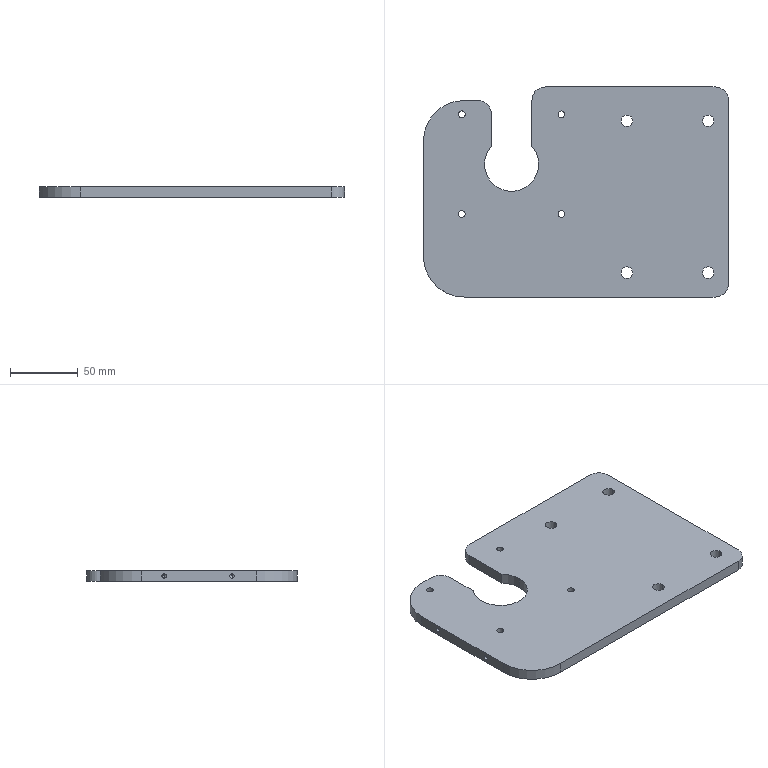Part | SolidWorks | features BaseBody 1 | 1 solid | 42 faces | box 225 x 155 x 8 mm | volume 249145 mm3 | cylinder 29 | plane 9 | cone 4 | commonest cylinder face diameters 5 x8 8.5 x8 3.3 x4 20 x4 40 x3 60 x2
STEP:
#1=CARTESIAN_POINT('',(-67.5,20.5,0.));
#2=VERTEX_POINT('',#1);
#3=CARTESIAN_POINT('',(-27.5,20.5,0.));
#4=VERTEX_POINT('',#3);
#5=CARTESIAN_POINT('',(-47.5,20.5,0.));
#6=DIRECTION('',(0.,0.,1.));
#7=DIRECTION('',(1.,0.,0.));
#8=AXIS2_PLACEMENT_3D('',#5,#6,#7);
#9=CIRCLE('',#8,20.);
#10=EDGE_CURVE('',#2,#4,#9,.T.);
#11=ORIENTED_EDGE('',*,*,#10,.F.);
#12=CARTESIAN_POINT('',(-67.5,20.5,8.));
#13=VERTEX_POINT('',#12);
#14=CARTESIAN_POINT('',(-67.5,20.5,0.));
#15=DIRECTION('',(0.,0.,1.));
#16=VECTOR('',#15,1000.);
#17=LINE('',#14,#16);
#18=EDGE_CURVE('',#2,#13,#17,.T.);
#19=ORIENTED_EDGE('',*,*,#18,.T.);
#20=CARTESIAN_POINT('',(-27.5,20.5,8.));
#21=VERTEX_POINT('',#20);
#22=CARTESIAN_POINT('',(-47.5,20.5,8.));
#23=DIRECTION('',(0.,0.,1.));
#24=DIRECTION('',(1.,0.,0.));
#25=AXIS2_PLACEMENT_3D('',#22,#23,#24);
#26=CIRCLE('',#25,20.);
#27=EDGE_CURVE('',#13,#21,#26,.T.);
#28=ORIENTED_EDGE('',*,*,#27,.T.);
#29=CARTESIAN_POINT('',(-27.5,20.5,0.));
#30=DIRECTION('',(0.,0.,1.));
#31=VECTOR('',#30,1000.);
#32=LINE('',#29,#31);
#33=EDGE_CURVE('',#4,#21,#32,.T.);
#34=ORIENTED_EDGE('',*,*,#33,.F.);
#35=EDGE_LOOP('',(#11,#19,#28,#34));
#36=FACE_OUTER_BOUND('',#35,.T.);
#37=CARTESIAN_POINT('',(-47.5,20.5,0.));
#38=DIRECTION('',(0.,0.,1.));
#39=DIRECTION('',(1.,0.,0.));
#40=AXIS2_PLACEMENT_3D('',#37,#38,#39);
#41=CYLINDRICAL_SURFACE('',#40,20.);
#42=ADVANCED_FACE('',(#36),#41,.F.);
#43=CARTESIAN_POINT('',(-32.5,33.729,0.));
#44=VERTEX_POINT('',#43);
#45=CARTESIAN_POINT('',(-47.5,20.5,0.));
#46=DIRECTION('',(0.,0.,1.));
#47=DIRECTION('',(1.,0.,0.));
#48=AXIS2_PLACEMENT_3D('',#45,#46,#47);
#49=CIRCLE('',#48,20.);
#50=EDGE_CURVE('',#4,#44,#49,.T.);
#51=ORIENTED_EDGE('',*,*,#50,.F.);
#52=ORIENTED_EDGE('',*,*,#33,.T.);
#53=CARTESIAN_POINT('',(-32.5,33.729,8.));
#54=VERTEX_POINT('',#53);
#55=CARTESIAN_POINT('',(-47.5,20.5,8.));
#56=DIRECTION('',(0.,0.,1.));
#57=DIRECTION('',(1.,0.,0.));
#58=AXIS2_PLACEMENT_3D('',#55,#56,#57);
#59=CIRCLE('',#58,20.);
#60=EDGE_CURVE('',#21,#54,#59,.T.);
#61=ORIENTED_EDGE('',*,*,#60,.T.);
#62=CARTESIAN_POINT('',(-32.5,33.729,8.));
#63=DIRECTION('',(0.,0.,-1.));
#64=VECTOR('',#63,1000.);
#65=LINE('',#62,#64);
#66=EDGE_CURVE('',#54,#44,#65,.T.);
#67=ORIENTED_EDGE('',*,*,#66,.T.);
#68=EDGE_LOOP('',(#51,#52,#61,#67));
#69=FACE_OUTER_BOUND('',#68,.T.);
#70=CARTESIAN_POINT('',(-47.5,20.5,0.));
#71=DIRECTION('',(0.,0.,1.));
#72=DIRECTION('',(1.,0.,0.));
#73=AXIS2_PLACEMENT_3D('',#70,#71,#72);
#74=CYLINDRICAL_SURFACE('',#73,20.);
#75=ADVANCED_FACE('',(#69),#74,.F.);
#76=CARTESIAN_POINT('',(33.25,52.5,8.));
#77=VERTEX_POINT('',#76);
#78=CARTESIAN_POINT('',(41.75,52.5,8.));
#79=VERTEX_POINT('',#78);
#80=CARTESIAN_POINT('',(37.5,52.5,8.));
#81=DIRECTION('',(0.,0.,1.));
#82=DIRECTION('',(-1.,0.,0.));
#83=AXIS2_PLACEMENT_3D('',#80,#81,#82);
#84=CIRCLE('',#83,4.25);
#85=EDGE_CURVE('',#77,#79,#84,.T.);
#86=ORIENTED_EDGE('',*,*,#85,.T.);
#87=CARTESIAN_POINT('',(41.75,52.5,0.));
#88=VERTEX_POINT('',#87);
#89=CARTESIAN_POINT('',(41.75,52.5,0.));
#90=DIRECTION('',(0.,0.,-1.));
#91=VECTOR('',#90,1000.);
#92=LINE('',#89,#91);
#93=EDGE_CURVE('',#79,#88,#92,.T.);
#94=ORIENTED_EDGE('',*,*,#93,.T.);
#95=CARTESIAN_POINT('',(33.25,52.5,0.));
#96=VERTEX_POINT('',#95);
#97=CARTESIAN_POINT('',(37.5,52.5,0.));
#98=DIRECTION('',(0.,0.,1.));
#99=DIRECTION('',(-1.,0.,0.));
#100=AXIS2_PLACEMENT_3D('',#97,#98,#99);
#101=CIRCLE('',#100,4.25);
#102=EDGE_CURVE('',#96,#88,#101,.T.);
#103=ORIENTED_EDGE('',*,*,#102,.F.);
#104=CARTESIAN_POINT('',(33.25,52.5,0.));
#105=DIRECTION('',(0.,0.,-1.));
#106=VECTOR('',#105,1000.);
#107=LINE('',#104,#106);
#108=EDGE_CURVE('',#77,#96,#107,.T.);
#109=ORIENTED_EDGE('',*,*,#108,.F.);
#110=EDGE_LOOP('',(#86,#94,#103,#109));
#111=FACE_OUTER_BOUND('',#110,.T.);
#112=CARTESIAN_POINT('',(37.5,52.5,0.));
#113=DIRECTION('',(0.,0.,-1.));
#114=DIRECTION('',(-1.,0.,0.));
#115=AXIS2_PLACEMENT_3D('',#112,#113,#114);
#116=CYLINDRICAL_SURFACE('',#115,4.25);
#117=ADVANCED_FACE('',(#111),#116,.F.);
#118=CARTESIAN_POINT('',(93.25,-59.5,8.));
#119=VERTEX_POINT('',#118);
#120=CARTESIAN_POINT('',(101.75,-59.5,8.));
#121=VERTEX_POINT('',#120);
#122=CARTESIAN_POINT('',(97.5,-59.5,8.));
#123=DIRECTION('',(0.,0.,1.));
#124=DIRECTION('',(-1.,0.,0.));
#125=AXIS2_PLACEMENT_3D('',#122,#123,#124);
#126=CIRCLE('',#125,4.25);
#127=EDGE_CURVE('',#119,#121,#126,.T.);
#128=ORIENTED_EDGE('',*,*,#127,.T.);
#129=CARTESIAN_POINT('',(101.75,-59.5,0.));
#130=VERTEX_POINT('',#129);
#131=CARTESIAN_POINT('',(101.75,-59.5,0.));
#132=DIRECTION('',(0.,0.,-1.));
#133=VECTOR('',#132,1000.);
#134=LINE('',#131,#133);
#135=EDGE_CURVE('',#121,#130,#134,.T.);
#136=ORIENTED_EDGE('',*,*,#135,.T.);
#137=CARTESIAN_POINT('',(93.25,-59.5,0.));
#138=VERTEX_POINT('',#137);
#139=CARTESIAN_POINT('',(97.5,-59.5,0.));
#140=DIRECTION('',(0.,0.,1.));
#141=DIRECTION('',(-1.,0.,0.));
#142=AXIS2_PLACEMENT_3D('',#139,#140,#141);
#143=CIRCLE('',#142,4.25);
#144=EDGE_CURVE('',#138,#130,#143,.T.);
#145=ORIENTED_EDGE('',*,*,#144,.F.);
#146=CARTESIAN_POINT('',(93.25,-59.5,0.));
#147=DIRECTION('',(0.,0.,-1.));
#148=VECTOR('',#147,1000.);
#149=LINE('',#146,#148);
#150=EDGE_CURVE('',#119,#138,#149,.T.);
#151=ORIENTED_EDGE('',*,*,#150,.F.);
#152=EDGE_LOOP('',(#128,#136,#145,#151));
#153=FACE_OUTER_BOUND('',#152,.T.);
#154=CARTESIAN_POINT('',(97.5,-59.5,0.));
#155=DIRECTION('',(0.,0.,-1.));
#156=DIRECTION('',(-1.,0.,0.));
#157=AXIS2_PLACEMENT_3D('',#154,#155,#156);
#158=CYLINDRICAL_SURFACE('',#157,4.25);
#159=ADVANCED_FACE('',(#153),#158,.F.);
#160=CARTESIAN_POINT('',(33.25,-59.5,8.));
#161=VERTEX_POINT('',#160);
#162=CARTESIAN_POINT('',(41.75,-59.5,8.));
#163=VERTEX_POINT('',#162);
#164=CARTESIAN_POINT('',(37.5,-59.5,8.));
#165=DIRECTION('',(0.,0.,1.));
#166=DIRECTION('',(-1.,0.,0.));
#167=AXIS2_PLACEMENT_3D('',#164,#165,#166);
#168=CIRCLE('',#167,4.25);
#169=EDGE_CURVE('',#161,#163,#168,.T.);
#170=ORIENTED_EDGE('',*,*,#169,.T.);
#171=CARTESIAN_POINT('',(41.75,-59.5,0.));
#172=VERTEX_POINT('',#171);
#173=CARTESIAN_POINT('',(41.75,-59.5,0.));
#174=DIRECTION('',(0.,0.,-1.));
#175=VECTOR('',#174,1000.);
#176=LINE('',#173,#175);
#177=EDGE_CURVE('',#163,#172,#176,.T.);
#178=ORIENTED_EDGE('',*,*,#177,.T.);
#179=CARTESIAN_POINT('',(33.25,-59.5,0.));
#180=VERTEX_POINT('',#179);
#181=CARTESIAN_POINT('',(37.5,-59.5,0.));
#182=DIRECTION('',(0.,0.,1.));
#183=DIRECTION('',(-1.,0.,0.));
#184=AXIS2_PLACEMENT_3D('',#181,#182,#183);
#185=CIRCLE('',#184,4.25);
#186=EDGE_CURVE('',#180,#172,#185,.T.);
#187=ORIENTED_EDGE('',*,*,#186,.F.);
#188=CARTESIAN_POINT('',(33.25,-59.5,0.));
#189=DIRECTION('',(0.,0.,-1.));
#190=VECTOR('',#189,1000.);
#191=LINE('',#188,#190);
#192=EDGE_CURVE('',#161,#180,#191,.T.);
#193=ORIENTED_EDGE('',*,*,#192,.F.);
#194=EDGE_LOOP('',(#170,#178,#187,#193));
#195=FACE_OUTER_BOUND('',#194,.T.);
#196=CARTESIAN_POINT('',(37.5,-59.5,0.));
#197=DIRECTION('',(0.,0.,-1.));
#198=DIRECTION('',(-1.,0.,0.));
#199=AXIS2_PLACEMENT_3D('',#196,#197,#198);
#200=CYLINDRICAL_SURFACE('',#199,4.25);
#201=ADVANCED_FACE('',(#195),#200,.F.);
#202=CARTESIAN_POINT('',(93.25,52.5,8.));
#203=VERTEX_POINT('',#202);
#204=CARTESIAN_POINT('',(101.75,52.5,8.));
#205=VERTEX_POINT('',#204);
#206=CARTESIAN_POINT('',(97.5,52.5,8.));
#207=DIRECTION('',(0.,0.,1.));
#208=DIRECTION('',(-1.,0.,0.));
#209=AXIS2_PLACEMENT_3D('',#206,#207,#208);
#210=CIRCLE('',#209,4.25);
#211=EDGE_CURVE('',#203,#205,#210,.T.);
#212=ORIENTED_EDGE('',*,*,#211,.T.);
#213=CARTESIAN_POINT('',(101.75,52.5,0.));
#214=VERTEX_POINT('',#213);
#215=CARTESIAN_POINT('',(101.75,52.5,0.));
#216=DIRECTION('',(0.,0.,-1.));
#217=VECTOR('',#216,1000.);
#218=LINE('',#215,#217);
#219=EDGE_CURVE('',#205,#214,#218,.T.);
#220=ORIENTED_EDGE('',*,*,#219,.T.);
#221=CARTESIAN_POINT('',(93.25,52.5,0.));
#222=VERTEX_POINT('',#221);
#223=CARTESIAN_POINT('',(97.5,52.5,0.));
#224=DIRECTION('',(0.,0.,1.));
#225=DIRECTION('',(-1.,0.,0.));
#226=AXIS2_PLACEMENT_3D('',#223,#224,#225);
#227=CIRCLE('',#226,4.25);
#228=EDGE_CURVE('',#222,#214,#227,.T.);
#229=ORIENTED_EDGE('',*,*,#228,.F.);
#230=CARTESIAN_POINT('',(93.25,52.5,0.));
#231=DIRECTION('',(0.,0.,-1.));
#232=VECTOR('',#231,1000.);
#233=LINE('',#230,#232);
#234=EDGE_CURVE('',#203,#222,#233,.T.);
#235=ORIENTED_EDGE('',*,*,#234,.F.);
#236=EDGE_LOOP('',(#212,#220,#229,#235));
#237=FACE_OUTER_BOUND('',#236,.T.);
#238=CARTESIAN_POINT('',(97.5,52.5,0.));
#239=DIRECTION('',(0.,0.,-1.));
#240=DIRECTION('',(-1.,0.,0.));
#241=AXIS2_PLACEMENT_3D('',#238,#239,#240);
#242=CYLINDRICAL_SURFACE('',#241,4.25);
#243=ADVANCED_FACE('',(#237),#242,.F.);
#244=CARTESIAN_POINT('',(-86.77,57.27,8.));
#245=VERTEX_POINT('',#244);
#246=CARTESIAN_POINT('',(-81.77,57.27,8.));
#247=VERTEX_POINT('',#246);
#248=CARTESIAN_POINT('',(-84.27,57.27,8.));
#249=DIRECTION('',(0.,0.,1.));
#250=DIRECTION('',(-1.,0.,0.));
#251=AXIS2_PLACEMENT_3D('',#248,#249,#250);
#252=CIRCLE('',#251,2.5);
#253=EDGE_CURVE('',#245,#247,#252,.T.);
#254=ORIENTED_EDGE('',*,*,#253,.T.);
#255=CARTESIAN_POINT('',(-81.77,57.27,0.));
#256=VERTEX_POINT('',#255);
#257=CARTESIAN_POINT('',(-81.77,57.27,0.));
#258=DIRECTION('',(0.,0.,-1.));
#259=VECTOR('',#258,1000.);
#260=LINE('',#257,#259);
#261=EDGE_CURVE('',#247,#256,#260,.T.);
#262=ORIENTED_EDGE('',*,*,#261,.T.);
#263=CARTESIAN_POINT('',(-86.77,57.27,0.));
#264=VERTEX_POINT('',#263);
#265=CARTESIAN_POINT('',(-84.27,57.27,0.));
#266=DIRECTION('',(0.,0.,1.));
#267=DIRECTION('',(-1.,0.,0.));
#268=AXIS2_PLACEMENT_3D('',#265,#266,#267);
#269=CIRCLE('',#268,2.5);
#270=EDGE_CURVE('',#264,#256,#269,.T.);
#271=ORIENTED_EDGE('',*,*,#270,.F.);
#272=CARTESIAN_POINT('',(-86.77,57.27,0.));
#273=DIRECTION('',(0.,0.,-1.));
#274=VECTOR('',#273,1000.);
#275=LINE('',#272,#274);
#276=EDGE_CURVE('',#245,#264,#275,.T.);
#277=ORIENTED_EDGE('',*,*,#276,.F.);
#278=EDGE_LOOP('',(#254,#262,#271,#277));
#279=FACE_OUTER_BOUND('',#278,.T.);
#280=CARTESIAN_POINT('',(-84.27,57.27,0.));
#281=DIRECTION('',(0.,0.,-1.));
#282=DIRECTION('',(-1.,0.,0.));
#283=AXIS2_PLACEMENT_3D('',#280,#281,#282);
#284=CYLINDRICAL_SURFACE('',#283,2.5);
#285=ADVANCED_FACE('',(#279),#284,.F.);
#286=CARTESIAN_POINT('',(-13.23,-16.27,8.));
#287=VERTEX_POINT('',#286);
#288=CARTESIAN_POINT('',(-8.23,-16.27,8.));
#289=VERTEX_POINT('',#288);
#290=CARTESIAN_POINT('',(-10.73,-16.27,8.));
#291=DIRECTION('',(0.,0.,1.));
#292=DIRECTION('',(-1.,0.,0.));
#293=AXIS2_PLACEMENT_3D('',#290,#291,#292);
#294=CIRCLE('',#293,2.5);
#295=EDGE_CURVE('',#287,#289,#294,.T.);
#296=ORIENTED_EDGE('',*,*,#295,.T.);
#297=CARTESIAN_POINT('',(-8.23,-16.27,0.));
#298=VERTEX_POINT('',#297);
#299=CARTESIAN_POINT('',(-8.23,-16.27,0.));
#300=DIRECTION('',(0.,0.,-1.));
#301=VECTOR('',#300,1000.);
#302=LINE('',#299,#301);
#303=EDGE_CURVE('',#289,#298,#302,.T.);
#304=ORIENTED_EDGE('',*,*,#303,.T.);
#305=CARTESIAN_POINT('',(-13.23,-16.27,0.));
#306=VERTEX_POINT('',#305);
#307=CARTESIAN_POINT('',(-10.73,-16.27,0.));
#308=DIRECTION('',(0.,0.,1.));
#309=DIRECTION('',(-1.,0.,0.));
#310=AXIS2_PLACEMENT_3D('',#307,#308,#309);
#311=CIRCLE('',#310,2.5);
#312=EDGE_CURVE('',#306,#298,#311,.T.);
#313=ORIENTED_EDGE('',*,*,#312,.F.);
#314=CARTESIAN_POINT('',(-13.23,-16.27,0.));
#315=DIRECTION('',(0.,0.,-1.));
#316=VECTOR('',#315,1000.);
#317=LINE('',#314,#316);
#318=EDGE_CURVE('',#287,#306,#317,.T.);
#319=ORIENTED_EDGE('',*,*,#318,.F.);
#320=EDGE_LOOP('',(#296,#304,#313,#319));
#321=FACE_OUTER_BOUND('',#320,.T.);
#322=CARTESIAN_POINT('',(-10.73,-16.27,0.));
#323=DIRECTION('',(0.,0.,-1.));
#324=DIRECTION('',(-1.,0.,0.));
#325=AXIS2_PLACEMENT_3D('',#322,#323,#324);
#326=CYLINDRICAL_SURFACE('',#325,2.5);
#327=ADVANCED_FACE('',(#321),#326,.F.);
#328=CARTESIAN_POINT('',(-13.23,57.27,8.));
#329=VERTEX_POINT('',#328);
#330=CARTESIAN_POINT('',(-8.23,57.27,8.));
#331=VERTEX_POINT('',#330);
#332=CARTESIAN_POINT('',(-10.73,57.27,8.));
#333=DIRECTION('',(0.,0.,1.));
#334=DIRECTION('',(-1.,0.,0.));
#335=AXIS2_PLACEMENT_3D('',#332,#333,#334);
#336=CIRCLE('',#335,2.5);
#337=EDGE_CURVE('',#329,#331,#336,.T.);
#338=ORIENTED_EDGE('',*,*,#337,.T.);
#339=CARTESIAN_POINT('',(-8.23,57.27,0.));
#340=VERTEX_POINT('',#339);
#341=CARTESIAN_POINT('',(-8.23,57.27,0.));
#342=DIRECTION('',(0.,0.,-1.));
#343=VECTOR('',#342,1000.);
#344=LINE('',#341,#343);
#345=EDGE_CURVE('',#331,#340,#344,.T.);
#346=ORIENTED_EDGE('',*,*,#345,.T.);
#347=CARTESIAN_POINT('',(-13.23,57.27,0.));
#348=VERTEX_POINT('',#347);
#349=CARTESIAN_POINT('',(-10.73,57.27,0.));
#350=DIRECTION('',(0.,0.,1.));
#351=DIRECTION('',(-1.,0.,0.));
#352=AXIS2_PLACEMENT_3D('',#349,#350,#351);
#353=CIRCLE('',#352,2.5);
#354=EDGE_CURVE('',#348,#340,#353,.T.);
#355=ORIENTED_EDGE('',*,*,#354,.F.);
#356=CARTESIAN_POINT('',(-13.23,57.27,0.));
#357=DIRECTION('',(0.,0.,-1.));
#358=VECTOR('',#357,1000.);
#359=LINE('',#356,#358);
#360=EDGE_CURVE('',#329,#348,#359,.T.);
#361=ORIENTED_EDGE('',*,*,#360,.F.);
#362=EDGE_LOOP('',(#338,#346,#355,#361));
#363=FACE_OUTER_BOUND('',#362,.T.);
#364=CARTESIAN_POINT('',(-10.73,57.27,0.));
#365=DIRECTION('',(0.,0.,-1.));
#366=DIRECTION('',(-1.,0.,0.));
#367=AXIS2_PLACEMENT_3D('',#364,#365,#366);
#368=CYLINDRICAL_SURFACE('',#367,2.5);
#369=ADVANCED_FACE('',(#363),#368,.F.);
#370=CARTESIAN_POINT('',(-86.77,-16.27,8.));
#371=VERTEX_POINT('',#370);
#372=CARTESIAN_POINT('',(-81.77,-16.27,8.));
#373=VERTEX_POINT('',#372);
#374=CARTESIAN_POINT('',(-84.27,-16.27,8.));
#375=DIRECTION('',(0.,0.,1.));
#376=DIRECTION('',(-1.,0.,0.));
#377=AXIS2_PLACEMENT_3D('',#374,#375,#376);
#378=CIRCLE('',#377,2.5);
#379=EDGE_CURVE('',#371,#373,#378,.T.);
#380=ORIENTED_EDGE('',*,*,#379,.T.);
#381=CARTESIAN_POINT('',(-81.77,-16.27,0.));
#382=VERTEX_POINT('',#381);
#383=CARTESIAN_POINT('',(-81.77,-16.27,0.));
#384=DIRECTION('',(0.,0.,-1.));
#385=VECTOR('',#384,1000.);
#386=LINE('',#383,#385);
#387=EDGE_CURVE('',#373,#382,#386,.T.);
#388=ORIENTED_EDGE('',*,*,#387,.T.);
#389=CARTESIAN_POINT('',(-86.77,-16.27,0.));
#390=VERTEX_POINT('',#389);
#391=CARTESIAN_POINT('',(-84.27,-16.27,0.));
#392=DIRECTION('',(0.,0.,1.));
#393=DIRECTION('',(-1.,0.,0.));
#394=AXIS2_PLACEMENT_3D('',#391,#392,#393);
#395=CIRCLE('',#394,2.5);
#396=EDGE_CURVE('',#390,#382,#395,.T.);
#397=ORIENTED_EDGE('',*,*,#396,.F.);
#398=CARTESIAN_POINT('',(-86.77,-16.27,0.));
#399=DIRECTION('',(0.,0.,-1.));
#400=VECTOR('',#399,1000.);
#401=LINE('',#398,#400);
#402=EDGE_CURVE('',#371,#390,#401,.T.);
#403=ORIENTED_EDGE('',*,*,#402,.F.);
#404=EDGE_LOOP('',(#380,#388,#397,#403));
#405=FACE_OUTER_BOUND('',#404,.T.);
#406=CARTESIAN_POINT('',(-84.27,-16.27,0.));
#407=DIRECTION('',(0.,0.,-1.));
#408=DIRECTION('',(-1.,0.,0.));
#409=AXIS2_PLACEMENT_3D('',#406,#407,#408);
#410=CYLINDRICAL_SURFACE('',#409,2.5);
#411=ADVANCED_FACE('',(#405),#410,.F.);
#412=CARTESIAN_POINT('',(-101.,20.5,2.35));
#413=VERTEX_POINT('',#412);
#414=CARTESIAN_POINT('',(-101.,20.5,5.65));
#415=VERTEX_POINT('',#414);
#416=CARTESIAN_POINT('',(-101.,20.5,4.));
#417=DIRECTION('',(-1.,0.,0.));
#418=DIRECTION('',(0.,0.,1.));
#419=AXIS2_PLACEMENT_3D('',#416,#417,#418);
#420=CIRCLE('',#419,1.65);
#421=EDGE_CURVE('',#413,#415,#420,.T.);
#422=ORIENTED_EDGE('',*,*,#421,.F.);
#423=CARTESIAN_POINT('',(-112.5,20.5,2.35));
#424=VERTEX_POINT('',#423);
#425=CARTESIAN_POINT('',(-112.5,20.5,2.35));
#426=DIRECTION('',(-1.,0.,0.));
#427=VECTOR('',#426,1000.);
#428=LINE('',#425,#427);
#429=EDGE_CURVE('',#413,#424,#428,.T.);
#430=ORIENTED_EDGE('',*,*,#429,.T.);
#431=CARTESIAN_POINT('',(-112.5,20.5,5.65));
#432=VERTEX_POINT('',#431);
#433=CARTESIAN_POINT('',(-112.5,20.5,4.));
#434=DIRECTION('',(-1.,0.,0.));
#435=DIRECTION('',(0.,0.,1.));
#436=AXIS2_PLACEMENT_3D('',#433,#434,#435);
#437=CIRCLE('',#436,1.65);
#438=EDGE_CURVE('',#424,#432,#437,.T.);
#439=ORIENTED_EDGE('',*,*,#438,.T.);
#440=CARTESIAN_POINT('',(-112.5,20.5,5.65));
#441=DIRECTION('',(-1.,0.,0.));
#442=VECTOR('',#441,1000.);
#443=LINE('',#440,#442);
#444=EDGE_CURVE('',#415,#432,#443,.T.);
#445=ORIENTED_EDGE('',*,*,#444,.F.);
#446=EDGE_LOOP('',(#422,#430,#439,#445));
#447=FACE_OUTER_BOUND('',#446,.T.);
#448=CARTESIAN_POINT('',(-112.5,20.5,4.));
#449=DIRECTION('',(-1.,0.,0.));
#450=DIRECTION('',(0.,0.,1.));
#451=AXIS2_PLACEMENT_3D('',#448,#449,#450);
#452=CYLINDRICAL_SURFACE('',#451,1.65);
#453=ADVANCED_FACE('',(#447),#452,.F.);
#454=CARTESIAN_POINT('',(-101.,-29.5,2.35));
#455=VERTEX_POINT('',#454);
#456=CARTESIAN_POINT('',(-101.,-29.5,5.65));
#457=VERTEX_POINT('',#456);
#458=CARTESIAN_POINT('',(-101.,-29.5,4.));
#459=DIRECTION('',(-1.,0.,0.));
#460=DIRECTION('',(0.,0.,1.));
#461=AXIS2_PLACEMENT_3D('',#458,#459,#460);
#462=CIRCLE('',#461,1.65);
#463=EDGE_CURVE('',#455,#457,#462,.T.);
#464=ORIENTED_EDGE('',*,*,#463,.F.);
#465=CARTESIAN_POINT('',(-112.5,-29.5,2.35));
#466=VERTEX_POINT('',#465);
#467=CARTESIAN_POINT('',(-112.5,-29.5,2.35));
#468=DIRECTION('',(-1.,0.,0.));
#469=VECTOR('',#468,1000.);
#470=LINE('',#467,#469);
#471=EDGE_CURVE('',#455,#466,#470,.T.);
#472=ORIENTED_EDGE('',*,*,#471,.T.);
#473=CARTESIAN_POINT('',(-112.5,-29.5,5.65));
#474=VERTEX_POINT('',#473);
#475=CARTESIAN_POINT('',(-112.5,-29.5,4.));
#476=DIRECTION('',(-1.,0.,0.));
#477=DIRECTION('',(0.,0.,1.));
#478=AXIS2_PLACEMENT_3D('',#475,#476,#477);
#479=CIRCLE('',#478,1.65);
#480=EDGE_CURVE('',#466,#474,#479,.T.);
#481=ORIENTED_EDGE('',*,*,#480,.T.);
#482=CARTESIAN_POINT('',(-112.5,-29.5,5.65));
#483=DIRECTION('',(-1.,0.,0.));
#484=VECTOR('',#483,1000.);
#485=LINE('',#482,#484);
#486=EDGE_CURVE('',#457,#474,#485,.T.);
#487=ORIENTED_EDGE('',*,*,#486,.F.);
#488=EDGE_LOOP('',(#464,#472,#481,#487));
#489=FACE_OUTER_BOUND('',#488,.T.);
#490=CARTESIAN_POINT('',(-112.5,-29.5,4.));
#491=DIRECTION('',(-1.,0.,0.));
#492=DIRECTION('',(0.,0.,1.));
#493=AXIS2_PLACEMENT_3D('',#490,#491,#492);
#494=CYLINDRICAL_SURFACE('',#493,1.65);
#495=ADVANCED_FACE('',(#489),#494,.F.);
#496=CARTESIAN_POINT('',(-100.009,20.5,4.));
#497=VERTEX_POINT('',#496);
#498=CARTESIAN_POINT('',(-101.,20.5,5.65));
#499=DIRECTION('',(-0.515,0.,0.8572));
#500=VECTOR('',#499,1000.);
#501=LINE('',#498,#500);
#502=EDGE_CURVE('',#497,#415,#501,.T.);
#503=ORIENTED_EDGE('',*,*,#502,.F.);
#504=CARTESIAN_POINT('',(-101.,20.5,2.35));
#505=DIRECTION('',(-0.515,0.,-0.8572));
#506=VECTOR('',#505,1000.);
#507=LINE('',#504,#506);
#508=EDGE_CURVE('',#497,#413,#507,.T.);
#509=ORIENTED_EDGE('',*,*,#508,.T.);
#510=ORIENTED_EDGE('',*,*,#421,.T.);
#511=EDGE_LOOP('',(#503,#509,#510));
#512=FACE_OUTER_BOUND('',#511,.T.);
#513=CARTESIAN_POINT('',(-101.,20.5,4.));
#514=DIRECTION('',(-1.,0.,0.));
#515=DIRECTION('',(0.,0.,1.));
#516=AXIS2_PLACEMENT_3D('',#513,#514,#515);
#517=CONICAL_SURFACE('',#516,1.65,1.03);
#518=ADVANCED_FACE('',(#512),#517,.F.);
#519=CARTESIAN_POINT('',(-100.009,-29.5,4.));
#520=VERTEX_POINT('',#519);
#521=CARTESIAN_POINT('',(-101.,-29.5,5.65));
#522=DIRECTION('',(-0.515,0.,0.8572));
#523=VECTOR('',#522,1000.);
#524=LINE('',#521,#523);
#525=EDGE_CURVE('',#520,#457,#524,.T.);
#526=ORIENTED_EDGE('',*,*,#525,.F.);
#527=CARTESIAN_POINT('',(-101.,-29.5,2.35));
#528=DIRECTION('',(-0.515,0.,-0.8572));
#529=VECTOR('',#528,1000.);
#530=LINE('',#527,#529);
#531=EDGE_CURVE('',#520,#455,#530,.T.);
#532=ORIENTED_EDGE('',*,*,#531,.T.);
#533=ORIENTED_EDGE('',*,*,#463,.T.);
#534=EDGE_LOOP('',(#526,#532,#533));
#535=FACE_OUTER_BOUND('',#534,.T.);
#536=CARTESIAN_POINT('',(-101.,-29.5,4.));
#537=DIRECTION('',(-1.,0.,0.));
#538=DIRECTION('',(0.,0.,1.));
#539=AXIS2_PLACEMENT_3D('',#536,#537,#538);
#540=CONICAL_SURFACE('',#539,1.65,1.03);
#541=ADVANCED_FACE('',(#535),#540,.F.);
#542=CARTESIAN_POINT('',(102.5,77.5,8.));
#543=VERTEX_POINT('',#542);
#544=CARTESIAN_POINT('',(112.5,67.5,8.));
#545=VERTEX_POINT('',#544);
#546=CARTESIAN_POINT('',(102.5,67.5,8.));
#547=DIRECTION('',(0.,0.,-1.));
#548=DIRECTION('',(-1.,0.,0.));
#549=AXIS2_PLACEMENT_3D('',#546,#547,#548);
#550=CIRCLE('',#549,10.);
#551=EDGE_CURVE('',#543,#545,#550,.T.);
#552=ORIENTED_EDGE('',*,*,#551,.F.);
#553=CARTESIAN_POINT('',(-22.5,77.5,8.));
#554=VERTEX_POINT('',#553);
#555=CARTESIAN_POINT('',(0.,77.5,8.));
#556=DIRECTION('',(1.,0.,0.));
#557=VECTOR('',#556,1000.);
#558=LINE('',#555,#557);
#559=EDGE_CURVE('',#554,#543,#558,.T.);
#560=ORIENTED_EDGE('',*,*,#559,.F.);
#561=CARTESIAN_POINT('',(-32.5,67.5,8.));
#562=VERTEX_POINT('',#561);
#563=CARTESIAN_POINT('',(-22.5,67.5,8.));
#564=DIRECTION('',(0.,0.,-1.));
#565=DIRECTION('',(1.,0.,0.));
#566=AXIS2_PLACEMENT_3D('',#563,#564,#565);
#567=CIRCLE('',#566,10.);
#568=EDGE_CURVE('',#562,#554,#567,.T.);
#569=ORIENTED_EDGE('',*,*,#568,.F.);
#570=CARTESIAN_POINT('',(-32.5,0.,8.));
#571=DIRECTION('',(0.,1.,0.));
#572=VECTOR('',#571,1000.);
#573=LINE('',#570,#572);
#574=EDGE_CURVE('',#54,#562,#573,.T.);
#575=ORIENTED_EDGE('',*,*,#574,.F.);
#576=ORIENTED_EDGE('',*,*,#60,.F.);
#577=ORIENTED_EDGE('',*,*,#27,.F.);
#578=CARTESIAN_POINT('',(-62.5,33.729,8.));
#579=VERTEX_POINT('',#578);
#580=CARTESIAN_POINT('',(-47.5,20.5,8.));
#581=DIRECTION('',(0.,0.,1.));
#582=DIRECTION('',(1.,0.,0.));
#583=AXIS2_PLACEMENT_3D('',#580,#581,#582);
#584=CIRCLE('',#583,20.);
#585=EDGE_CURVE('',#579,#13,#584,.T.);
#586=ORIENTED_EDGE('',*,*,#585,.F.);
#587=CARTESIAN_POINT('',(-62.5,57.5,8.));
#588=VERTEX_POINT('',#587);
#589=CARTESIAN_POINT('',(-62.5,0.,8.));
#590=DIRECTION('',(0.,-1.,0.));
#591=VECTOR('',#590,1000.);
#592=LINE('',#589,#591);
#593=EDGE_CURVE('',#588,#579,#592,.T.);
#594=ORIENTED_EDGE('',*,*,#593,.F.);
#595=CARTESIAN_POINT('',(-72.5,67.5,8.));
#596=VERTEX_POINT('',#595);
#597=CARTESIAN_POINT('',(-72.5,57.5,8.));
#598=DIRECTION('',(0.,0.,-1.));
#599=DIRECTION('',(1.,0.,0.));
#600=AXIS2_PLACEMENT_3D('',#597,#598,#599);
#601=CIRCLE('',#600,10.);
#602=EDGE_CURVE('',#596,#588,#601,.T.);
#603=ORIENTED_EDGE('',*,*,#602,.F.);
#604=CARTESIAN_POINT('',(-82.5,67.5,8.));
#605=VERTEX_POINT('',#604);
#606=CARTESIAN_POINT('',(0.,67.5,8.));
#607=DIRECTION('',(1.,0.,0.));
#608=VECTOR('',#607,1000.);
#609=LINE('',#606,#608);
#610=EDGE_CURVE('',#605,#596,#609,.T.);
#611=ORIENTED_EDGE('',*,*,#610,.F.);
#612=CARTESIAN_POINT('',(-112.5,37.5,8.));
#613=VERTEX_POINT('',#612);
#614=CARTESIAN_POINT('',(-82.5,37.5,8.));
#615=DIRECTION('',(0.,0.,-1.));
#616=DIRECTION('',(1.,0.,0.));
#617=AXIS2_PLACEMENT_3D('',#614,#615,#616);
#618=CIRCLE('',#617,30.);
#619=EDGE_CURVE('',#613,#605,#618,.T.);
#620=ORIENTED_EDGE('',*,*,#619,.F.);
#621=CARTESIAN_POINT('',(-112.5,-47.5,8.));
#622=VERTEX_POINT('',#621);
#623=CARTESIAN_POINT('',(-112.5,0.,8.));
#624=DIRECTION('',(0.,1.,0.));
#625=VECTOR('',#624,1000.);
#626=LINE('',#623,#625);
#627=EDGE_CURVE('',#622,#613,#626,.T.);
#628=ORIENTED_EDGE('',*,*,#627,.F.);
#629=CARTESIAN_POINT('',(-82.5,-77.5,8.));
#630=VERTEX_POINT('',#629);
#631=CARTESIAN_POINT('',(-82.5,-47.5,8.));
#632=DIRECTION('',(0.,0.,-1.));
#633=DIRECTION('',(-1.,0.,0.));
#634=AXIS2_PLACEMENT_3D('',#631,#632,#633);
#635=CIRCLE('',#634,30.);
#636=EDGE_CURVE('',#630,#622,#635,.T.);
#637=ORIENTED_EDGE('',*,*,#636,.F.);
#638=CARTESIAN_POINT('',(102.5,-77.5,8.));
#639=VERTEX_POINT('',#638);
#640=CARTESIAN_POINT('',(0.,-77.5,8.));
#641=DIRECTION('',(-1.,0.,0.));
#642=VECTOR('',#641,1000.);
#643=LINE('',#640,#642);
#644=EDGE_CURVE('',#639,#630,#643,.T.);
#645=ORIENTED_EDGE('',*,*,#644,.F.);
#646=CARTESIAN_POINT('',(112.5,-67.5,8.));
#647=VERTEX_POINT('',#646);
#648=CARTESIAN_POINT('',(102.5,-67.5,8.));
#649=DIRECTION('',(0.,0.,-1.));
#650=DIRECTION('',(-1.,0.,0.));
#651=AXIS2_PLACEMENT_3D('',#648,#649,#650);
#652=CIRCLE('',#651,10.);
#653=EDGE_CURVE('',#647,#639,#652,.T.);
#654=ORIENTED_EDGE('',*,*,#653,.F.);
#655=CARTESIAN_POINT('',(112.5,0.,8.));
#656=DIRECTION('',(0.,-1.,0.));
#657=VECTOR('',#656,1000.);
#658=LINE('',#655,#657);
#659=EDGE_CURVE('',#545,#647,#658,.T.);
#660=ORIENTED_EDGE('',*,*,#659,.F.);
#661=EDGE_LOOP('',(#552,#560,#569,#575,#576,#577,#586,#594,#603,#611,#620,#628,#637,#645,#654,#660));
#662=FACE_OUTER_BOUND('',#661,.T.);
#663=ORIENTED_EDGE('',*,*,#85,.F.);
#664=CARTESIAN_POINT('',(37.5,52.5,8.));
#665=DIRECTION('',(0.,0.,1.));
#666=DIRECTION('',(-1.,0.,0.));
#667=AXIS2_PLACEMENT_3D('',#664,#665,#666);
#668=CIRCLE('',#667,4.25);
#669=EDGE_CURVE('',#79,#77,#668,.T.);
#670=ORIENTED_EDGE('',*,*,#669,.F.);
#671=EDGE_LOOP('',(#663,#670));
#672=FACE_BOUND('',#671,.T.);
#673=ORIENTED_EDGE('',*,*,#127,.F.);
#674=CARTESIAN_POINT('',(97.5,-59.5,8.));
#675=DIRECTION('',(0.,0.,1.));
#676=DIRECTION('',(-1.,0.,0.));
#677=AXIS2_PLACEMENT_3D('',#674,#675,#676);
#678=CIRCLE('',#677,4.25);
#679=EDGE_CURVE('',#121,#119,#678,.T.);
#680=ORIENTED_EDGE('',*,*,#679,.F.);
#681=EDGE_LOOP('',(#673,#680));
#682=FACE_BOUND('',#681,.T.);
#683=ORIENTED_EDGE('',*,*,#169,.F.);
#684=CARTESIAN_POINT('',(37.5,-59.5,8.));
#685=DIRECTION('',(0.,0.,1.));
#686=DIRECTION('',(-1.,0.,0.));
#687=AXIS2_PLACEMENT_3D('',#684,#685,#686);
#688=CIRCLE('',#687,4.25);
#689=EDGE_CURVE('',#163,#161,#688,.T.);
#690=ORIENTED_EDGE('',*,*,#689,.F.);
#691=EDGE_LOOP('',(#683,#690));
#692=FACE_BOUND('',#691,.T.);
#693=ORIENTED_EDGE('',*,*,#211,.F.);
#694=CARTESIAN_POINT('',(97.5,52.5,8.));
#695=DIRECTION('',(0.,0.,1.));
#696=DIRECTION('',(-1.,0.,0.));
#697=AXIS2_PLACEMENT_3D('',#694,#695,#696);
#698=CIRCLE('',#697,4.25);
#699=EDGE_CURVE('',#205,#203,#698,.T.);
#700=ORIENTED_EDGE('',*,*,#699,.F.);
#701=EDGE_LOOP('',(#693,#700));
#702=FACE_BOUND('',#701,.T.);
#703=ORIENTED_EDGE('',*,*,#253,.F.);
#704=CARTESIAN_POINT('',(-84.27,57.27,8.));
#705=DIRECTION('',(0.,0.,1.));
#706=DIRECTION('',(-1.,0.,0.));
#707=AXIS2_PLACEMENT_3D('',#704,#705,#706);
#708=CIRCLE('',#707,2.5);
#709=EDGE_CURVE('',#247,#245,#708,.T.);
#710=ORIENTED_EDGE('',*,*,#709,.F.);
#711=EDGE_LOOP('',(#703,#710));
#712=FACE_BOUND('',#711,.T.);
#713=ORIENTED_EDGE('',*,*,#295,.F.);
#714=CARTESIAN_POINT('',(-10.73,-16.27,8.));
#715=DIRECTION('',(0.,0.,1.));
#716=DIRECTION('',(-1.,0.,0.));
#717=AXIS2_PLACEMENT_3D('',#714,#715,#716);
#718=CIRCLE('',#717,2.5);
#719=EDGE_CURVE('',#289,#287,#718,.T.);
#720=ORIENTED_EDGE('',*,*,#719,.F.);
#721=EDGE_LOOP('',(#713,#720));
#722=FACE_BOUND('',#721,.T.);
#723=ORIENTED_EDGE('',*,*,#337,.F.);
#724=CARTESIAN_POINT('',(-10.73,57.27,8.));
#725=DIRECTION('',(0.,0.,1.));
#726=DIRECTION('',(-1.,0.,0.));
#727=AXIS2_PLACEMENT_3D('',#724,#725,#726);
#728=CIRCLE('',#727,2.5);
#729=EDGE_CURVE('',#331,#329,#728,.T.);
#730=ORIENTED_EDGE('',*,*,#729,.F.);
#731=EDGE_LOOP('',(#723,#730));
#732=FACE_BOUND('',#731,.T.);
#733=ORIENTED_EDGE('',*,*,#379,.F.);
#734=CARTESIAN_POINT('',(-84.27,-16.27,8.));
#735=DIRECTION('',(0.,0.,1.));
#736=DIRECTION('',(-1.,0.,0.));
#737=AXIS2_PLACEMENT_3D('',#734,#735,#736);
#738=CIRCLE('',#737,2.5);
#739=EDGE_CURVE('',#373,#371,#738,.T.);
#740=ORIENTED_EDGE('',*,*,#739,.F.);
#741=EDGE_LOOP('',(#733,#740));
#742=FACE_BOUND('',#741,.T.);
#743=CARTESIAN_POINT('',(0.,0.,8.));
#744=DIRECTION('',(0.,0.,-1.));
#745=DIRECTION('',(-1.,0.,0.));
#746=AXIS2_PLACEMENT_3D('',#743,#744,#745);
#747=PLANE('',#746);
#748=ADVANCED_FACE('',(#662,#672,#682,#692,#702,#712,#722,#732,#742),#747,.F.);
#749=CARTESIAN_POINT('',(112.5,67.5,0.));
#750=VERTEX_POINT('',#749);
#751=CARTESIAN_POINT('',(112.5,67.5,8.));
#752=DIRECTION('',(0.,0.,-1.));
#753=VECTOR('',#752,1000.);
#754=LINE('',#751,#753);
#755=EDGE_CURVE('',#545,#750,#754,.T.);
#756=ORIENTED_EDGE('',*,*,#755,.F.);
#757=ORIENTED_EDGE('',*,*,#659,.T.);
#758=CARTESIAN_POINT('',(112.5,-67.5,0.));
#759=VERTEX_POINT('',#758);
#760=CARTESIAN_POINT('',(112.5,-67.5,8.));
#761=DIRECTION('',(0.,0.,1.));
#762=VECTOR('',#761,1000.);
#763=LINE('',#760,#762);
#764=EDGE_CURVE('',#759,#647,#763,.T.);
#765=ORIENTED_EDGE('',*,*,#764,.F.);
#766=CARTESIAN_POINT('',(112.5,-77.5,0.));
#767=DIRECTION('',(0.,-1.,0.));
#768=VECTOR('',#767,1000.);
#769=LINE('',#766,#768);
#770=EDGE_CURVE('',#750,#759,#769,.T.);
#771=ORIENTED_EDGE('',*,*,#770,.F.);
#772=EDGE_LOOP('',(#756,#757,#765,#771));
#773=FACE_OUTER_BOUND('',#772,.T.);
#774=CARTESIAN_POINT('',(112.5,-77.5,8.));
#775=DIRECTION('',(-1.,0.,0.));
#776=DIRECTION('',(0.,0.,1.));
#777=AXIS2_PLACEMENT_3D('',#774,#775,#776);
#778=PLANE('',#777);
#779=ADVANCED_FACE('',(#773),#778,.F.);
#780=CARTESIAN_POINT('',(102.5,77.5,0.));
#781=VERTEX_POINT('',#780);
#782=CARTESIAN_POINT('',(102.5,67.5,0.));
#783=DIRECTION('',(0.,0.,1.));
#784=DIRECTION('',(-1.,0.,0.));
#785=AXIS2_PLACEMENT_3D('',#782,#783,#784);
#786=CIRCLE('',#785,10.);
#787=EDGE_CURVE('',#750,#781,#786,.T.);
#788=ORIENTED_EDGE('',*,*,#787,.T.);
#789=CARTESIAN_POINT('',(102.5,77.5,8.));
#790=DIRECTION('',(0.,0.,1.));
#791=VECTOR('',#790,1000.);
#792=LINE('',#789,#791);
#793=EDGE_CURVE('',#781,#543,#792,.T.);
#794=ORIENTED_EDGE('',*,*,#793,.T.);
#795=ORIENTED_EDGE('',*,*,#551,.T.);
#796=ORIENTED_EDGE('',*,*,#755,.T.);
#797=EDGE_LOOP('',(#788,#794,#795,#796));
#798=FACE_OUTER_BOUND('',#797,.T.);
#799=CARTESIAN_POINT('',(102.5,67.5,8.));
#800=DIRECTION('',(0.,0.,-1.));
#801=DIRECTION('',(-1.,0.,0.));
#802=AXIS2_PLACEMENT_3D('',#799,#800,#801);
#803=CYLINDRICAL_SURFACE('',#802,10.);
#804=ADVANCED_FACE('',(#798),#803,.T.);
#805=ORIENTED_EDGE('',*,*,#793,.F.);
#806=CARTESIAN_POINT('',(-22.5,77.5,0.));
#807=VERTEX_POINT('',#806);
#808=CARTESIAN_POINT('',(-112.5,77.5,0.));
#809=DIRECTION('',(1.,0.,0.));
#810=VECTOR('',#809,1000.);
#811=LINE('',#808,#810);
#812=EDGE_CURVE('',#807,#781,#811,.T.);
#813=ORIENTED_EDGE('',*,*,#812,.F.);
#814=CARTESIAN_POINT('',(-22.5,77.5,8.));
#815=DIRECTION('',(0.,0.,-1.));
#816=VECTOR('',#815,1000.);
#817=LINE('',#814,#816);
#818=EDGE_CURVE('',#554,#807,#817,.T.);
#819=ORIENTED_EDGE('',*,*,#818,.F.);
#820=ORIENTED_EDGE('',*,*,#559,.T.);
#821=EDGE_LOOP('',(#805,#813,#819,#820));
#822=FACE_OUTER_BOUND('',#821,.T.);
#823=CARTESIAN_POINT('',(-112.5,77.5,8.));
#824=DIRECTION('',(0.,-1.,0.));
#825=DIRECTION('',(0.,0.,-1.));
#826=AXIS2_PLACEMENT_3D('',#823,#824,#825);
#827=PLANE('',#826);
#828=ADVANCED_FACE('',(#822),#827,.F.);
#829=ORIENTED_EDGE('',*,*,#568,.T.);
#830=ORIENTED_EDGE('',*,*,#818,.T.);
#831=CARTESIAN_POINT('',(-32.5,67.5,0.));
#832=VERTEX_POINT('',#831);
#833=CARTESIAN_POINT('',(-22.5,67.5,0.));
#834=DIRECTION('',(0.,0.,1.));
#835=DIRECTION('',(1.,0.,0.));
#836=AXIS2_PLACEMENT_3D('',#833,#834,#835);
#837=CIRCLE('',#836,10.);
#838=EDGE_CURVE('',#807,#832,#837,.T.);
#839=ORIENTED_EDGE('',*,*,#838,.T.);
#840=CARTESIAN_POINT('',(-32.5,67.5,8.));
#841=DIRECTION('',(0.,0.,1.));
#842=VECTOR('',#841,1000.);
#843=LINE('',#840,#842);
#844=EDGE_CURVE('',#832,#562,#843,.T.);
#845=ORIENTED_EDGE('',*,*,#844,.T.);
#846=EDGE_LOOP('',(#829,#830,#839,#845));
#847=FACE_OUTER_BOUND('',#846,.T.);
#848=CARTESIAN_POINT('',(-22.5,67.5,8.));
#849=DIRECTION('',(0.,0.,1.));
#850=DIRECTION('',(1.,0.,0.));
#851=AXIS2_PLACEMENT_3D('',#848,#849,#850);
#852=CYLINDRICAL_SURFACE('',#851,10.);
#853=ADVANCED_FACE('',(#847),#852,.T.);
#854=ORIENTED_EDGE('',*,*,#844,.F.);
#855=CARTESIAN_POINT('',(-32.5,82.09,0.));
#856=DIRECTION('',(0.,1.,0.));
#857=VECTOR('',#856,1000.);
#858=LINE('',#855,#857);
#859=EDGE_CURVE('',#44,#832,#858,.T.);
#860=ORIENTED_EDGE('',*,*,#859,.F.);
#861=ORIENTED_EDGE('',*,*,#66,.F.);
#862=ORIENTED_EDGE('',*,*,#574,.T.);
#863=EDGE_LOOP('',(#854,#860,#861,#862));
#864=FACE_OUTER_BOUND('',#863,.T.);
#865=CARTESIAN_POINT('',(-32.5,82.09,8.));
#866=DIRECTION('',(1.,0.,0.));
#867=DIRECTION('',(0.,1.,0.));
#868=AXIS2_PLACEMENT_3D('',#865,#866,#867);
#869=PLANE('',#868);
#870=ADVANCED_FACE('',(#864),#869,.F.);
#871=ORIENTED_EDGE('',*,*,#18,.F.);
#872=CARTESIAN_POINT('',(-62.5,33.729,0.));
#873=VERTEX_POINT('',#872);
#874=CARTESIAN_POINT('',(-47.5,20.5,0.));
#875=DIRECTION('',(0.,0.,1.));
#876=DIRECTION('',(1.,0.,0.));
#877=AXIS2_PLACEMENT_3D('',#874,#875,#876);
#878=CIRCLE('',#877,20.);
#879=EDGE_CURVE('',#873,#2,#878,.T.);
#880=ORIENTED_EDGE('',*,*,#879,.F.);
#881=CARTESIAN_POINT('',(-62.5,33.729,0.));
#882=DIRECTION('',(0.,0.,-1.));
#883=VECTOR('',#882,1000.);
#884=LINE('',#881,#883);
#885=EDGE_CURVE('',#579,#873,#884,.T.);
#886=ORIENTED_EDGE('',*,*,#885,.F.);
#887=ORIENTED_EDGE('',*,*,#585,.T.);
#888=EDGE_LOOP('',(#871,#880,#886,#887));
#889=FACE_OUTER_BOUND('',#888,.T.);
#890=CARTESIAN_POINT('',(-47.5,20.5,0.));
#891=DIRECTION('',(0.,0.,1.));
#892=DIRECTION('',(1.,0.,0.));
#893=AXIS2_PLACEMENT_3D('',#890,#891,#892);
#894=CYLINDRICAL_SURFACE('',#893,20.);
#895=ADVANCED_FACE('',(#889),#894,.F.);
#896=CARTESIAN_POINT('',(-62.5,57.5,0.));
#897=VERTEX_POINT('',#896);
#898=CARTESIAN_POINT('',(-62.5,57.5,8.));
#899=DIRECTION('',(0.,0.,-1.));
#900=VECTOR('',#899,1000.);
#901=LINE('',#898,#900);
#902=EDGE_CURVE('',#588,#897,#901,.T.);
#903=ORIENTED_EDGE('',*,*,#902,.F.);
#904=ORIENTED_EDGE('',*,*,#593,.T.);
#905=ORIENTED_EDGE('',*,*,#885,.T.);
#906=CARTESIAN_POINT('',(-62.5,82.09,0.));
#907=DIRECTION('',(0.,-1.,0.));
#908=VECTOR('',#907,1000.);
#909=LINE('',#906,#908);
#910=EDGE_CURVE('',#897,#873,#909,.T.);
#911=ORIENTED_EDGE('',*,*,#910,.F.);
#912=EDGE_LOOP('',(#903,#904,#905,#911));
#913=FACE_OUTER_BOUND('',#912,.T.);
#914=CARTESIAN_POINT('',(-62.5,82.09,8.));
#915=DIRECTION('',(-1.,0.,0.));
#916=DIRECTION('',(0.,0.,1.));
#917=AXIS2_PLACEMENT_3D('',#914,#915,#916);
#918=PLANE('',#917);
#919=ADVANCED_FACE('',(#913),#918,.F.);
#920=ORIENTED_EDGE('',*,*,#602,.T.);
#921=ORIENTED_EDGE('',*,*,#902,.T.);
#922=CARTESIAN_POINT('',(-72.5,67.5,0.));
#923=VERTEX_POINT('',#922);
#924=CARTESIAN_POINT('',(-72.5,57.5,0.));
#925=DIRECTION('',(0.,0.,1.));
#926=DIRECTION('',(1.,0.,0.));
#927=AXIS2_PLACEMENT_3D('',#924,#925,#926);
#928=CIRCLE('',#927,10.);
#929=EDGE_CURVE('',#897,#923,#928,.T.);
#930=ORIENTED_EDGE('',*,*,#929,.T.);
#931=CARTESIAN_POINT('',(-72.5,67.5,8.));
#932=DIRECTION('',(0.,0.,1.));
#933=VECTOR('',#932,1000.);
#934=LINE('',#931,#933);
#935=EDGE_CURVE('',#923,#596,#934,.T.);
#936=ORIENTED_EDGE('',*,*,#935,.T.);
#937=EDGE_LOOP('',(#920,#921,#930,#936));
#938=FACE_OUTER_BOUND('',#937,.T.);
#939=CARTESIAN_POINT('',(-72.5,57.5,8.));
#940=DIRECTION('',(0.,0.,1.));
#941=DIRECTION('',(1.,0.,0.));
#942=AXIS2_PLACEMENT_3D('',#939,#940,#941);
#943=CYLINDRICAL_SURFACE('',#942,10.);
#944=ADVANCED_FACE('',(#938),#943,.T.);
#945=ORIENTED_EDGE('',*,*,#935,.F.);
#946=CARTESIAN_POINT('',(-82.5,67.5,0.));
#947=VERTEX_POINT('',#946);
#948=CARTESIAN_POINT('',(-62.5,67.5,0.));
#949=DIRECTION('',(1.,0.,0.));
#950=VECTOR('',#949,1000.);
#951=LINE('',#948,#950);
#952=EDGE_CURVE('',#947,#923,#951,.T.);
#953=ORIENTED_EDGE('',*,*,#952,.F.);
#954=CARTESIAN_POINT('',(-82.5,67.5,0.));
#955=DIRECTION('',(0.,0.,-1.));
#956=VECTOR('',#955,1000.);
#957=LINE('',#954,#956);
#958=EDGE_CURVE('',#605,#947,#957,.T.);
#959=ORIENTED_EDGE('',*,*,#958,.F.);
#960=ORIENTED_EDGE('',*,*,#610,.T.);
#961=EDGE_LOOP('',(#945,#953,#959,#960));
#962=FACE_OUTER_BOUND('',#961,.T.);
#963=CARTESIAN_POINT('',(-62.5,67.5,0.));
#964=DIRECTION('',(0.,-1.,0.));
#965=DIRECTION('',(0.,0.,-1.));
#966=AXIS2_PLACEMENT_3D('',#963,#964,#965);
#967=PLANE('',#966);
#968=ADVANCED_FACE('',(#962),#967,.F.);
#969=ORIENTED_EDGE('',*,*,#619,.T.);
#970=ORIENTED_EDGE('',*,*,#958,.T.);
#971=CARTESIAN_POINT('',(-112.5,37.5,0.));
#972=VERTEX_POINT('',#971);
#973=CARTESIAN_POINT('',(-82.5,37.5,0.));
#974=DIRECTION('',(0.,0.,1.));
#975=DIRECTION('',(1.,0.,0.));
#976=AXIS2_PLACEMENT_3D('',#973,#974,#975);
#977=CIRCLE('',#976,30.);
#978=EDGE_CURVE('',#947,#972,#977,.T.);
#979=ORIENTED_EDGE('',*,*,#978,.T.);
#980=CARTESIAN_POINT('',(-112.5,37.5,0.));
#981=DIRECTION('',(0.,0.,1.));
#982=VECTOR('',#981,1000.);
#983=LINE('',#980,#982);
#984=EDGE_CURVE('',#972,#613,#983,.T.);
#985=ORIENTED_EDGE('',*,*,#984,.T.);
#986=EDGE_LOOP('',(#969,#970,#979,#985));
#987=FACE_OUTER_BOUND('',#986,.T.);
#988=CARTESIAN_POINT('',(-82.5,37.5,0.));
#989=DIRECTION('',(0.,0.,1.));
#990=DIRECTION('',(1.,0.,0.));
#991=AXIS2_PLACEMENT_3D('',#988,#989,#990);
#992=CYLINDRICAL_SURFACE('',#991,30.);
#993=ADVANCED_FACE('',(#987),#992,.T.);
#994=CARTESIAN_POINT('',(-112.5,-47.5,0.));
#995=VERTEX_POINT('',#994);
#996=CARTESIAN_POINT('',(-112.5,-47.5,8.));
#997=DIRECTION('',(0.,0.,-1.));
#998=VECTOR('',#997,1000.);
#999=LINE('',#996,#998);
#1000=EDGE_CURVE('',#622,#995,#999,.T.);
#1001=ORIENTED_EDGE('',*,*,#1000,.F.);
#1002=ORIENTED_EDGE('',*,*,#627,.T.);
#1003=ORIENTED_EDGE('',*,*,#984,.F.);
#1004=CARTESIAN_POINT('',(-112.5,-77.5,0.));
#1005=DIRECTION('',(0.,1.,0.));
#1006=VECTOR('',#1005,1000.);
#1007=LINE('',#1004,#1006);
#1008=EDGE_CURVE('',#995,#972,#1007,.T.);
#1009=ORIENTED_EDGE('',*,*,#1008,.F.);
#1010=EDGE_LOOP('',(#1001,#1002,#1003,#1009));
#1011=FACE_OUTER_BOUND('',#1010,.T.);
#1012=CARTESIAN_POINT('',(-112.5,20.5,4.));
#1013=DIRECTION('',(-1.,0.,0.));
#1014=DIRECTION('',(0.,0.,1.));
#1015=AXIS2_PLACEMENT_3D('',#1012,#1013,#1014);
#1016=CIRCLE('',#1015,1.65);
#1017=EDGE_CURVE('',#432,#424,#1016,.T.);
#1018=ORIENTED_EDGE('',*,*,#1017,.F.);
#1019=ORIENTED_EDGE('',*,*,#438,.F.);
#1020=EDGE_LOOP('',(#1018,#1019));
#1021=FACE_BOUND('',#1020,.T.);
#1022=CARTESIAN_POINT('',(-112.5,-29.5,4.));
#1023=DIRECTION('',(-1.,0.,0.));
#1024=DIRECTION('',(0.,0.,1.));
#1025=AXIS2_PLACEMENT_3D('',#1022,#1023,#1024);
#1026=CIRCLE('',#1025,1.65);
#1027=EDGE_CURVE('',#474,#466,#1026,.T.);
#1028=ORIENTED_EDGE('',*,*,#1027,.F.);
#1029=ORIENTED_EDGE('',*,*,#480,.F.);
#1030=EDGE_LOOP('',(#1028,#1029));
#1031=FACE_BOUND('',#1030,.T.);
#1032=CARTESIAN_POINT('',(-112.5,-77.5,8.));
#1033=DIRECTION('',(1.,0.,0.));
#1034=DIRECTION('',(0.,0.,-1.));
#1035=AXIS2_PLACEMENT_3D('',#1032,#1033,#1034);
#1036=PLANE('',#1035);
#1037=ADVANCED_FACE('',(#1011,#1021,#1031),#1036,.F.);
#1038=CARTESIAN_POINT('',(-82.5,-77.5,0.));
#1039=VERTEX_POINT('',#1038);
#1040=CARTESIAN_POINT('',(-82.5,-47.5,0.));
#1041=DIRECTION('',(0.,0.,1.));
#1042=DIRECTION('',(-1.,0.,0.));
#1043=AXIS2_PLACEMENT_3D('',#1040,#1041,#1042);
#1044=CIRCLE('',#1043,30.);
#1045=EDGE_CURVE('',#995,#1039,#1044,.T.);
#1046=ORIENTED_EDGE('',*,*,#1045,.T.);
#1047=CARTESIAN_POINT('',(-82.5,-77.5,8.));
#1048=DIRECTION('',(0.,0.,1.));
#1049=VECTOR('',#1048,1000.);
#1050=LINE('',#1047,#1049);
#1051=EDGE_CURVE('',#1039,#630,#1050,.T.);
#1052=ORIENTED_EDGE('',*,*,#1051,.T.);
#1053=ORIENTED_EDGE('',*,*,#636,.T.);
#1054=ORIENTED_EDGE('',*,*,#1000,.T.);
#1055=EDGE_LOOP('',(#1046,#1052,#1053,#1054));
#1056=FACE_OUTER_BOUND('',#1055,.T.);
#1057=CARTESIAN_POINT('',(-82.5,-47.5,8.));
#1058=DIRECTION('',(0.,0.,-1.));
#1059=DIRECTION('',(-1.,0.,0.));
#1060=AXIS2_PLACEMENT_3D('',#1057,#1058,#1059);
#1061=CYLINDRICAL_SURFACE('',#1060,30.);
#1062=ADVANCED_FACE('',(#1056),#1061,.T.);
#1063=CARTESIAN_POINT('',(102.5,-77.5,0.));
#1064=VERTEX_POINT('',#1063);
#1065=CARTESIAN_POINT('',(102.5,-77.5,8.));
#1066=DIRECTION('',(0.,0.,-1.));
#1067=VECTOR('',#1066,1000.);
#1068=LINE('',#1065,#1067);
#1069=EDGE_CURVE('',#639,#1064,#1068,.T.);
#1070=ORIENTED_EDGE('',*,*,#1069,.F.);
#1071=ORIENTED_EDGE('',*,*,#644,.T.);
#1072=ORIENTED_EDGE('',*,*,#1051,.F.);
#1073=CARTESIAN_POINT('',(-112.5,-77.5,0.));
#1074=DIRECTION('',(-1.,0.,0.));
#1075=VECTOR('',#1074,1000.);
#1076=LINE('',#1073,#1075);
#1077=EDGE_CURVE('',#1064,#1039,#1076,.T.);
#1078=ORIENTED_EDGE('',*,*,#1077,.F.);
#1079=EDGE_LOOP('',(#1070,#1071,#1072,#1078));
#1080=FACE_OUTER_BOUND('',#1079,.T.);
#1081=CARTESIAN_POINT('',(-112.5,-77.5,8.));
#1082=DIRECTION('',(0.,1.,0.));
#1083=DIRECTION('',(0.,0.,1.));
#1084=AXIS2_PLACEMENT_3D('',#1081,#1082,#1083);
#1085=PLANE('',#1084);
#1086=ADVANCED_FACE('',(#1080),#1085,.F.);
#1087=CARTESIAN_POINT('',(102.5,-67.5,0.));
#1088=DIRECTION('',(0.,0.,1.));
#1089=DIRECTION('',(-1.,0.,0.));
#1090=AXIS2_PLACEMENT_3D('',#1087,#1088,#1089);
#1091=CIRCLE('',#1090,10.);
#1092=EDGE_CURVE('',#1064,#759,#1091,.T.);
#1093=ORIENTED_EDGE('',*,*,#1092,.T.);
#1094=ORIENTED_EDGE('',*,*,#764,.T.);
#1095=ORIENTED_EDGE('',*,*,#653,.T.);
#1096=ORIENTED_EDGE('',*,*,#1069,.T.);
#1097=EDGE_LOOP('',(#1093,#1094,#1095,#1096));
#1098=FACE_OUTER_BOUND('',#1097,.T.);
#1099=CARTESIAN_POINT('',(102.5,-67.5,8.));
#1100=DIRECTION('',(0.,0.,-1.));
#1101=DIRECTION('',(-1.,0.,0.));
#1102=AXIS2_PLACEMENT_3D('',#1099,#1100,#1101);
#1103=CYLINDRICAL_SURFACE('',#1102,10.);
#1104=ADVANCED_FACE('',(#1098),#1103,.T.);
#1105=ORIENTED_EDGE('',*,*,#93,.F.);
#1106=ORIENTED_EDGE('',*,*,#669,.T.);
#1107=ORIENTED_EDGE('',*,*,#108,.T.);
#1108=CARTESIAN_POINT('',(37.5,52.5,0.));
#1109=DIRECTION('',(0.,0.,1.));
#1110=DIRECTION('',(-1.,0.,0.));
#1111=AXIS2_PLACEMENT_3D('',#1108,#1109,#1110);
#1112=CIRCLE('',#1111,4.25);
#1113=EDGE_CURVE('',#88,#96,#1112,.T.);
#1114=ORIENTED_EDGE('',*,*,#1113,.F.);
#1115=EDGE_LOOP('',(#1105,#1106,#1107,#1114));
#1116=FACE_OUTER_BOUND('',#1115,.T.);
#1117=CARTESIAN_POINT('',(37.5,52.5,0.));
#1118=DIRECTION('',(0.,0.,-1.));
#1119=DIRECTION('',(-1.,0.,0.));
#1120=AXIS2_PLACEMENT_3D('',#1117,#1118,#1119);
#1121=CYLINDRICAL_SURFACE('',#1120,4.25);
#1122=ADVANCED_FACE('',(#1116),#1121,.F.);
#1123=ORIENTED_EDGE('',*,*,#135,.F.);
#1124=ORIENTED_EDGE('',*,*,#679,.T.);
#1125=ORIENTED_EDGE('',*,*,#150,.T.);
#1126=CARTESIAN_POINT('',(97.5,-59.5,0.));
#1127=DIRECTION('',(0.,0.,1.));
#1128=DIRECTION('',(-1.,0.,0.));
#1129=AXIS2_PLACEMENT_3D('',#1126,#1127,#1128);
#1130=CIRCLE('',#1129,4.25);
#1131=EDGE_CURVE('',#130,#138,#1130,.T.);
#1132=ORIENTED_EDGE('',*,*,#1131,.F.);
#1133=EDGE_LOOP('',(#1123,#1124,#1125,#1132));
#1134=FACE_OUTER_BOUND('',#1133,.T.);
#1135=CARTESIAN_POINT('',(97.5,-59.5,0.));
#1136=DIRECTION('',(0.,0.,-1.));
#1137=DIRECTION('',(-1.,0.,0.));
#1138=AXIS2_PLACEMENT_3D('',#1135,#1136,#1137);
#1139=CYLINDRICAL_SURFACE('',#1138,4.25);
#1140=ADVANCED_FACE('',(#1134),#1139,.F.);
#1141=ORIENTED_EDGE('',*,*,#177,.F.);
#1142=ORIENTED_EDGE('',*,*,#689,.T.);
#1143=ORIENTED_EDGE('',*,*,#192,.T.);
#1144=CARTESIAN_POINT('',(37.5,-59.5,0.));
#1145=DIRECTION('',(0.,0.,1.));
#1146=DIRECTION('',(-1.,0.,0.));
#1147=AXIS2_PLACEMENT_3D('',#1144,#1145,#1146);
#1148=CIRCLE('',#1147,4.25);
#1149=EDGE_CURVE('',#172,#180,#1148,.T.);
#1150=ORIENTED_EDGE('',*,*,#1149,.F.);
#1151=EDGE_LOOP('',(#1141,#1142,#1143,#1150));
#1152=FACE_OUTER_BOUND('',#1151,.T.);
#1153=CARTESIAN_POINT('',(37.5,-59.5,0.));
#1154=DIRECTION('',(0.,0.,-1.));
#1155=DIRECTION('',(-1.,0.,0.));
#1156=AXIS2_PLACEMENT_3D('',#1153,#1154,#1155);
#1157=CYLINDRICAL_SURFACE('',#1156,4.25);
#1158=ADVANCED_FACE('',(#1152),#1157,.F.);
#1159=ORIENTED_EDGE('',*,*,#219,.F.);
#1160=ORIENTED_EDGE('',*,*,#699,.T.);
#1161=ORIENTED_EDGE('',*,*,#234,.T.);
#1162=CARTESIAN_POINT('',(97.5,52.5,0.));
#1163=DIRECTION('',(0.,0.,1.));
#1164=DIRECTION('',(-1.,0.,0.));
#1165=AXIS2_PLACEMENT_3D('',#1162,#1163,#1164);
#1166=CIRCLE('',#1165,4.25);
#1167=EDGE_CURVE('',#214,#222,#1166,.T.);
#1168=ORIENTED_EDGE('',*,*,#1167,.F.);
#1169=EDGE_LOOP('',(#1159,#1160,#1161,#1168));
#1170=FACE_OUTER_BOUND('',#1169,.T.);
#1171=CARTESIAN_POINT('',(97.5,52.5,0.));
#1172=DIRECTION('',(0.,0.,-1.));
#1173=DIRECTION('',(-1.,0.,0.));
#1174=AXIS2_PLACEMENT_3D('',#1171,#1172,#1173);
#1175=CYLINDRICAL_SURFACE('',#1174,4.25);
#1176=ADVANCED_FACE('',(#1170),#1175,.F.);
#1177=ORIENTED_EDGE('',*,*,#261,.F.);
#1178=ORIENTED_EDGE('',*,*,#709,.T.);
#1179=ORIENTED_EDGE('',*,*,#276,.T.);
#1180=CARTESIAN_POINT('',(-84.27,57.27,0.));
#1181=DIRECTION('',(0.,0.,1.));
#1182=DIRECTION('',(-1.,0.,0.));
#1183=AXIS2_PLACEMENT_3D('',#1180,#1181,#1182);
#1184=CIRCLE('',#1183,2.5);
#1185=EDGE_CURVE('',#256,#264,#1184,.T.);
#1186=ORIENTED_EDGE('',*,*,#1185,.F.);
#1187=EDGE_LOOP('',(#1177,#1178,#1179,#1186));
#1188=FACE_OUTER_BOUND('',#1187,.T.);
#1189=CARTESIAN_POINT('',(-84.27,57.27,0.));
#1190=DIRECTION('',(0.,0.,-1.));
#1191=DIRECTION('',(-1.,0.,0.));
#1192=AXIS2_PLACEMENT_3D('',#1189,#1190,#1191);
#1193=CYLINDRICAL_SURFACE('',#1192,2.5);
#1194=ADVANCED_FACE('',(#1188),#1193,.F.);
#1195=ORIENTED_EDGE('',*,*,#303,.F.);
#1196=ORIENTED_EDGE('',*,*,#719,.T.);
#1197=ORIENTED_EDGE('',*,*,#318,.T.);
#1198=CARTESIAN_POINT('',(-10.73,-16.27,0.));
#1199=DIRECTION('',(0.,0.,1.));
#1200=DIRECTION('',(-1.,0.,0.));
#1201=AXIS2_PLACEMENT_3D('',#1198,#1199,#1200);
#1202=CIRCLE('',#1201,2.5);
#1203=EDGE_CURVE('',#298,#306,#1202,.T.);
#1204=ORIENTED_EDGE('',*,*,#1203,.F.);
#1205=EDGE_LOOP('',(#1195,#1196,#1197,#1204));
#1206=FACE_OUTER_BOUND('',#1205,.T.);
#1207=CARTESIAN_POINT('',(-10.73,-16.27,0.));
#1208=DIRECTION('',(0.,0.,-1.));
#1209=DIRECTION('',(-1.,0.,0.));
#1210=AXIS2_PLACEMENT_3D('',#1207,#1208,#1209);
#1211=CYLINDRICAL_SURFACE('',#1210,2.5);
#1212=ADVANCED_FACE('',(#1206),#1211,.F.);
#1213=ORIENTED_EDGE('',*,*,#345,.F.);
#1214=ORIENTED_EDGE('',*,*,#729,.T.);
#1215=ORIENTED_EDGE('',*,*,#360,.T.);
#1216=CARTESIAN_POINT('',(-10.73,57.27,0.));
#1217=DIRECTION('',(0.,0.,1.));
#1218=DIRECTION('',(-1.,0.,0.));
#1219=AXIS2_PLACEMENT_3D('',#1216,#1217,#1218);
#1220=CIRCLE('',#1219,2.5);
#1221=EDGE_CURVE('',#340,#348,#1220,.T.);
#1222=ORIENTED_EDGE('',*,*,#1221,.F.);
#1223=EDGE_LOOP('',(#1213,#1214,#1215,#1222));
#1224=FACE_OUTER_BOUND('',#1223,.T.);
#1225=CARTESIAN_POINT('',(-10.73,57.27,0.));
#1226=DIRECTION('',(0.,0.,-1.));
#1227=DIRECTION('',(-1.,0.,0.));
#1228=AXIS2_PLACEMENT_3D('',#1225,#1226,#1227);
#1229=CYLINDRICAL_SURFACE('',#1228,2.5);
#1230=ADVANCED_FACE('',(#1224),#1229,.F.);
#1231=ORIENTED_EDGE('',*,*,#387,.F.);
#1232=ORIENTED_EDGE('',*,*,#739,.T.);
#1233=ORIENTED_EDGE('',*,*,#402,.T.);
#1234=CARTESIAN_POINT('',(-84.27,-16.27,0.));
#1235=DIRECTION('',(0.,0.,1.));
#1236=DIRECTION('',(-1.,0.,0.));
#1237=AXIS2_PLACEMENT_3D('',#1234,#1235,#1236);
#1238=CIRCLE('',#1237,2.5);
#1239=EDGE_CURVE('',#382,#390,#1238,.T.);
#1240=ORIENTED_EDGE('',*,*,#1239,.F.);
#1241=EDGE_LOOP('',(#1231,#1232,#1233,#1240));
#1242=FACE_OUTER_BOUND('',#1241,.T.);
#1243=CARTESIAN_POINT('',(-84.27,-16.27,0.));
#1244=DIRECTION('',(0.,0.,-1.));
#1245=DIRECTION('',(-1.,0.,0.));
#1246=AXIS2_PLACEMENT_3D('',#1243,#1244,#1245);
#1247=CYLINDRICAL_SURFACE('',#1246,2.5);
#1248=ADVANCED_FACE('',(#1242),#1247,.F.);
#1249=ORIENTED_EDGE('',*,*,#102,.T.);
#1250=ORIENTED_EDGE('',*,*,#1113,.T.);
#1251=EDGE_LOOP('',(#1249,#1250));
#1252=FACE_BOUND('',#1251,.T.);
#1253=ORIENTED_EDGE('',*,*,#144,.T.);
#1254=ORIENTED_EDGE('',*,*,#1131,.T.);
#1255=EDGE_LOOP('',(#1253,#1254));
#1256=FACE_BOUND('',#1255,.T.);
#1257=ORIENTED_EDGE('',*,*,#186,.T.);
#1258=ORIENTED_EDGE('',*,*,#1149,.T.);
#1259=EDGE_LOOP('',(#1257,#1258));
#1260=FACE_BOUND('',#1259,.T.);
#1261=ORIENTED_EDGE('',*,*,#228,.T.);
#1262=ORIENTED_EDGE('',*,*,#1167,.T.);
#1263=EDGE_LOOP('',(#1261,#1262));
#1264=FACE_BOUND('',#1263,.T.);
#1265=ORIENTED_EDGE('',*,*,#270,.T.);
#1266=ORIENTED_EDGE('',*,*,#1185,.T.);
#1267=EDGE_LOOP('',(#1265,#1266));
#1268=FACE_BOUND('',#1267,.T.);
#1269=ORIENTED_EDGE('',*,*,#312,.T.);
#1270=ORIENTED_EDGE('',*,*,#1203,.T.);
#1271=EDGE_LOOP('',(#1269,#1270));
#1272=FACE_BOUND('',#1271,.T.);
#1273=ORIENTED_EDGE('',*,*,#354,.T.);
#1274=ORIENTED_EDGE('',*,*,#1221,.T.);
#1275=EDGE_LOOP('',(#1273,#1274));
#1276=FACE_BOUND('',#1275,.T.);
#1277=ORIENTED_EDGE('',*,*,#396,.T.);
#1278=ORIENTED_EDGE('',*,*,#1239,.T.);
#1279=EDGE_LOOP('',(#1277,#1278));
#1280=FACE_BOUND('',#1279,.T.);
#1281=ORIENTED_EDGE('',*,*,#859,.T.);
#1282=ORIENTED_EDGE('',*,*,#838,.F.);
#1283=ORIENTED_EDGE('',*,*,#812,.T.);
#1284=ORIENTED_EDGE('',*,*,#787,.F.);
#1285=ORIENTED_EDGE('',*,*,#770,.T.);
#1286=ORIENTED_EDGE('',*,*,#1092,.F.);
#1287=ORIENTED_EDGE('',*,*,#1077,.T.);
#1288=ORIENTED_EDGE('',*,*,#1045,.F.);
#1289=ORIENTED_EDGE('',*,*,#1008,.T.);
#1290=ORIENTED_EDGE('',*,*,#978,.F.);
#1291=ORIENTED_EDGE('',*,*,#952,.T.);
#1292=ORIENTED_EDGE('',*,*,#929,.F.);
#1293=ORIENTED_EDGE('',*,*,#910,.T.);
#1294=ORIENTED_EDGE('',*,*,#879,.T.);
#1295=ORIENTED_EDGE('',*,*,#10,.T.);
#1296=ORIENTED_EDGE('',*,*,#50,.T.);
#1297=EDGE_LOOP('',(#1281,#1282,#1283,#1284,#1285,#1286,#1287,#1288,#1289,#1290,#1291,#1292,#1293,#1294,#1295,#1296));
#1298=FACE_OUTER_BOUND('',#1297,.T.);
#1299=CARTESIAN_POINT('',(0.,0.,0.));
#1300=DIRECTION('',(0.,0.,-1.));
#1301=DIRECTION('',(-1.,0.,0.));
#1302=AXIS2_PLACEMENT_3D('',#1299,#1300,#1301);
#1303=PLANE('',#1302);
#1304=ADVANCED_FACE('',(#1252,#1256,#1260,#1264,#1268,#1272,#1276,#1280,#1298),#1303,.T.);
#1305=ORIENTED_EDGE('',*,*,#429,.F.);
#1306=CARTESIAN_POINT('',(-101.,20.5,4.));
#1307=DIRECTION('',(-1.,0.,0.));
#1308=DIRECTION('',(0.,0.,1.));
#1309=AXIS2_PLACEMENT_3D('',#1306,#1307,#1308);
#1310=CIRCLE('',#1309,1.65);
#1311=EDGE_CURVE('',#415,#413,#1310,.T.);
#1312=ORIENTED_EDGE('',*,*,#1311,.F.);
#1313=ORIENTED_EDGE('',*,*,#444,.T.);
#1314=ORIENTED_EDGE('',*,*,#1017,.T.);
#1315=EDGE_LOOP('',(#1305,#1312,#1313,#1314));
#1316=FACE_OUTER_BOUND('',#1315,.T.);
#1317=CARTESIAN_POINT('',(-112.5,20.5,4.));
#1318=DIRECTION('',(-1.,0.,0.));
#1319=DIRECTION('',(0.,0.,1.));
#1320=AXIS2_PLACEMENT_3D('',#1317,#1318,#1319);
#1321=CYLINDRICAL_SURFACE('',#1320,1.65);
#1322=ADVANCED_FACE('',(#1316),#1321,.F.);
#1323=ORIENTED_EDGE('',*,*,#471,.F.);
#1324=CARTESIAN_POINT('',(-101.,-29.5,4.));
#1325=DIRECTION('',(-1.,0.,0.));
#1326=DIRECTION('',(0.,0.,1.));
#1327=AXIS2_PLACEMENT_3D('',#1324,#1325,#1326);
#1328=CIRCLE('',#1327,1.65);
#1329=EDGE_CURVE('',#457,#455,#1328,.T.);
#1330=ORIENTED_EDGE('',*,*,#1329,.F.);
#1331=ORIENTED_EDGE('',*,*,#486,.T.);
#1332=ORIENTED_EDGE('',*,*,#1027,.T.);
#1333=EDGE_LOOP('',(#1323,#1330,#1331,#1332));
#1334=FACE_OUTER_BOUND('',#1333,.T.);
#1335=CARTESIAN_POINT('',(-112.5,-29.5,4.));
#1336=DIRECTION('',(-1.,0.,0.));
#1337=DIRECTION('',(0.,0.,1.));
#1338=AXIS2_PLACEMENT_3D('',#1335,#1336,#1337);
#1339=CYLINDRICAL_SURFACE('',#1338,1.65);
#1340=ADVANCED_FACE('',(#1334),#1339,.F.);
#1341=ORIENTED_EDGE('',*,*,#508,.F.);
#1342=ORIENTED_EDGE('',*,*,#502,.T.);
#1343=ORIENTED_EDGE('',*,*,#1311,.T.);
#1344=EDGE_LOOP('',(#1341,#1342,#1343));
#1345=FACE_OUTER_BOUND('',#1344,.T.);
#1346=CARTESIAN_POINT('',(-101.,20.5,4.));
#1347=DIRECTION('',(-1.,0.,0.));
#1348=DIRECTION('',(0.,0.,1.));
#1349=AXIS2_PLACEMENT_3D('',#1346,#1347,#1348);
#1350=CONICAL_SURFACE('',#1349,1.65,1.03);
#1351=ADVANCED_FACE('',(#1345),#1350,.F.);
#1352=ORIENTED_EDGE('',*,*,#531,.F.);
#1353=ORIENTED_EDGE('',*,*,#525,.T.);
#1354=ORIENTED_EDGE('',*,*,#1329,.T.);
#1355=EDGE_LOOP('',(#1352,#1353,#1354));
#1356=FACE_OUTER_BOUND('',#1355,.T.);
#1357=CARTESIAN_POINT('',(-101.,-29.5,4.));
#1358=DIRECTION('',(-1.,0.,0.));
#1359=DIRECTION('',(0.,0.,1.));
#1360=AXIS2_PLACEMENT_3D('',#1357,#1358,#1359);
#1361=CONICAL_SURFACE('',#1360,1.65,1.03);
#1362=ADVANCED_FACE('',(#1356),#1361,.F.);
#1363=CLOSED_SHELL('',(#42,#75,#117,#159,#201,#243,#285,#327,#369,#411,#453,#495,#518,#541,#748,#779,#804,#828,#853,#870,#895,#919,#944,#968,#993,#1037,#1062,#1086,#1104,#1122,#1140,#1158,#1176,#1194,#1212,#1230,#1248,#1304,#1322,#1340,#1351,#1362));
#1364=MANIFOLD_SOLID_BREP('',#1363);
#1365=CARTESIAN_POINT('',(0.,0.,0.));
#1366=DIRECTION('',(0.,0.,1.));
#1367=DIRECTION('',(1.,0.,0.));
#1368=AXIS2_PLACEMENT_3D('',#1365,#1366,#1367);
#1369=(LENGTH_UNIT()NAMED_UNIT(*)SI_UNIT(.MILLI.,.METRE.));
#1370=UNCERTAINTY_MEASURE_WITH_UNIT(LENGTH_MEASURE(0.00001),#1369,'','');
#1371=(NAMED_UNIT(*)PLANE_ANGLE_UNIT()SI_UNIT($,.RADIAN.));
#1372=(NAMED_UNIT(*)SI_UNIT($,.STERADIAN.)SOLID_ANGLE_UNIT());
#1373=(GEOMETRIC_REPRESENTATION_CONTEXT(3)GLOBAL_UNCERTAINTY_ASSIGNED_CONTEXT((#1370))GLOBAL_UNIT_ASSIGNED_CONTEXT((#1369,#1371,#1372))REPRESENTATION_CONTEXT('',''));
#1374=ADVANCED_BREP_SHAPE_REPRESENTATION('',(#1364,#1368),#1373);